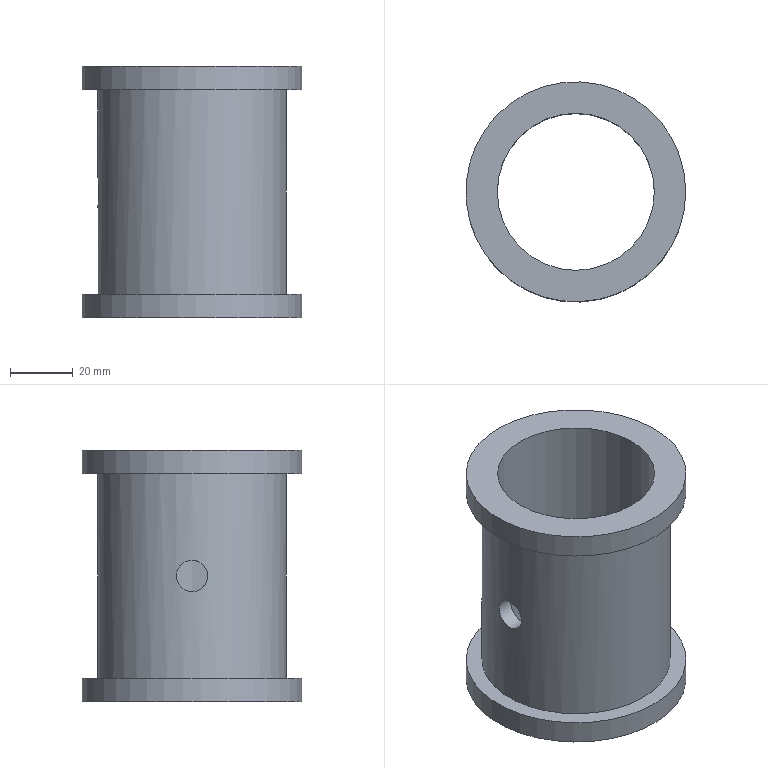Part | NX | features CYLINDER 5, DATUM_CSYS 1 | 1 solid | 9 faces | box 70 x 70 x 80 mm | volume 84036 mm3 | cylinder 5 | plane 4 | commonest cylinder face diameters 70 x2 10 x1 50 x1 60 x1
STEP:
#1=CARTESIAN_POINT('',(-30.,0.,45.));
#2=VERTEX_POINT('',#1);
#3=CARTESIAN_POINT('',(-29.791,-3.922,43.915));
#4=CARTESIAN_POINT('',(-30.104,0.0009284,45.542));
#5=CARTESIAN_POINT('',(-29.792,3.919,43.916));
#6=CARTESIAN_POINT('',(-29.475,5.54,40.005));
#7=CARTESIAN_POINT('',(-29.791,3.919,36.082));
#8=CARTESIAN_POINT('',(-30.104,0.001467,34.46));
#9=CARTESIAN_POINT('',(-29.792,-3.914,36.078));
#10=CARTESIAN_POINT('',(-29.475,-5.541,39.996));
#11=CARTESIAN_POINT('',(-29.791,-3.922,43.915));
#12=CARTESIAN_POINT('',(-30.104,0.0009284,45.542));
#13=CARTESIAN_POINT('',(-29.792,3.919,43.916));
#14=B_SPLINE_CURVE_WITH_KNOTS('',3,(#3,#4,#5,#6,#7,#8,#9,#10,#11,#12,#13),.UNSPECIFIED.,.T.,.F.,(1,1,1,1,1,1,1,1,1,1,1,1,1,1,1),(-0.01174,-0.007829,-0.003914,0.,0.003914,0.007829,0.01174,0.01566,0.01957,0.02349,0.0274,0.03132,0.03523,0.03914,0.04306),.UNSPECIFIED.);
#15=EDGE_CURVE('',#2,#2,#14,.T.);
#16=ORIENTED_EDGE('',*,*,#15,.F.);
#17=EDGE_LOOP('',(#16));
#18=FACE_BOUND('',#17,.T.);
#19=CARTESIAN_POINT('',(-30.,0.,72.5));
#20=VERTEX_POINT('',#19);
#21=CARTESIAN_POINT('',(0.,0.,72.5));
#22=DIRECTION('',(0.,0.,-1.));
#23=DIRECTION('',(-1.,0.,0.));
#24=AXIS2_PLACEMENT_3D('',#21,#22,#23);
#25=CIRCLE('',#24,30.);
#26=EDGE_CURVE('',#20,#20,#25,.F.);
#27=ORIENTED_EDGE('',*,*,#26,.F.);
#28=EDGE_LOOP('',(#27));
#29=FACE_BOUND('',#28,.T.);
#30=CARTESIAN_POINT('',(30.,0.,7.5));
#31=VERTEX_POINT('',#30);
#32=CARTESIAN_POINT('',(0.,0.,7.5));
#33=DIRECTION('',(0.,0.,1.));
#34=DIRECTION('',(1.,0.,0.));
#35=AXIS2_PLACEMENT_3D('',#32,#33,#34);
#36=CIRCLE('',#35,30.);
#37=EDGE_CURVE('',#31,#31,#36,.F.);
#38=ORIENTED_EDGE('',*,*,#37,.F.);
#39=EDGE_LOOP('',(#38));
#40=FACE_BOUND('',#39,.T.);
#41=CARTESIAN_POINT('',(0.,0.,0.));
#42=DIRECTION('',(0.,0.,1.));
#43=DIRECTION('',(1.,0.,0.));
#44=AXIS2_PLACEMENT_3D('',#41,#42,#43);
#45=CYLINDRICAL_SURFACE('',#44,30.);
#46=ADVANCED_FACE('',(#18,#29,#40),#45,.T.);
#47=ORIENTED_EDGE('',*,*,#37,.T.);
#48=EDGE_LOOP('',(#47));
#49=FACE_BOUND('',#48,.T.);
#50=CARTESIAN_POINT('',(35.,0.,7.5));
#51=VERTEX_POINT('',#50);
#52=CARTESIAN_POINT('',(0.,0.,7.5));
#53=DIRECTION('',(0.,0.,-1.));
#54=DIRECTION('',(1.,0.,0.));
#55=AXIS2_PLACEMENT_3D('',#52,#53,#54);
#56=CIRCLE('',#55,35.);
#57=EDGE_CURVE('',#51,#51,#56,.T.);
#58=ORIENTED_EDGE('',*,*,#57,.F.);
#59=EDGE_LOOP('',(#58));
#60=FACE_BOUND('',#59,.T.);
#61=CARTESIAN_POINT('',(0.,0.,7.5));
#62=DIRECTION('',(0.,0.,1.));
#63=DIRECTION('',(1.,0.,0.));
#64=AXIS2_PLACEMENT_3D('',#61,#62,#63);
#65=PLANE('',#64);
#66=ADVANCED_FACE('',(#49,#60),#65,.T.);
#67=ORIENTED_EDGE('',*,*,#57,.T.);
#68=EDGE_LOOP('',(#67));
#69=FACE_BOUND('',#68,.T.);
#70=CARTESIAN_POINT('',(35.,0.,0.));
#71=VERTEX_POINT('',#70);
#72=CARTESIAN_POINT('',(0.,0.,0.));
#73=DIRECTION('',(0.,0.,1.));
#74=DIRECTION('',(1.,0.,0.));
#75=AXIS2_PLACEMENT_3D('',#72,#73,#74);
#76=CIRCLE('',#75,35.);
#77=EDGE_CURVE('',#71,#71,#76,.T.);
#78=ORIENTED_EDGE('',*,*,#77,.T.);
#79=EDGE_LOOP('',(#78));
#80=FACE_BOUND('',#79,.T.);
#81=CARTESIAN_POINT('',(0.,0.,0.));
#82=DIRECTION('',(0.,0.,1.));
#83=DIRECTION('',(1.,0.,0.));
#84=AXIS2_PLACEMENT_3D('',#81,#82,#83);
#85=CYLINDRICAL_SURFACE('',#84,35.);
#86=ADVANCED_FACE('',(#69,#80),#85,.T.);
#87=CARTESIAN_POINT('',(25.,0.,0.));
#88=VERTEX_POINT('',#87);
#89=CARTESIAN_POINT('',(0.,0.,0.));
#90=DIRECTION('',(0.,0.,1.));
#91=DIRECTION('',(1.,0.,0.));
#92=AXIS2_PLACEMENT_3D('',#89,#90,#91);
#93=CIRCLE('',#92,25.);
#94=EDGE_CURVE('',#88,#88,#93,.T.);
#95=ORIENTED_EDGE('',*,*,#94,.T.);
#96=EDGE_LOOP('',(#95));
#97=FACE_BOUND('',#96,.T.);
#98=ORIENTED_EDGE('',*,*,#77,.F.);
#99=EDGE_LOOP('',(#98));
#100=FACE_BOUND('',#99,.T.);
#101=CARTESIAN_POINT('',(0.,0.,0.));
#102=DIRECTION('',(0.,0.,-1.));
#103=DIRECTION('',(-1.,0.,0.));
#104=AXIS2_PLACEMENT_3D('',#101,#102,#103);
#105=PLANE('',#104);
#106=ADVANCED_FACE('',(#97,#100),#105,.T.);
#107=ORIENTED_EDGE('',*,*,#26,.T.);
#108=EDGE_LOOP('',(#107));
#109=FACE_BOUND('',#108,.T.);
#110=CARTESIAN_POINT('',(35.,0.,72.5));
#111=VERTEX_POINT('',#110);
#112=CARTESIAN_POINT('',(0.,0.,72.5));
#113=DIRECTION('',(0.,0.,1.));
#114=DIRECTION('',(1.,0.,0.));
#115=AXIS2_PLACEMENT_3D('',#112,#113,#114);
#116=CIRCLE('',#115,35.);
#117=EDGE_CURVE('',#111,#111,#116,.T.);
#118=ORIENTED_EDGE('',*,*,#117,.F.);
#119=EDGE_LOOP('',(#118));
#120=FACE_BOUND('',#119,.T.);
#121=CARTESIAN_POINT('',(0.,0.,72.5));
#122=DIRECTION('',(0.,0.,-1.));
#123=DIRECTION('',(-1.,0.,0.));
#124=AXIS2_PLACEMENT_3D('',#121,#122,#123);
#125=PLANE('',#124);
#126=ADVANCED_FACE('',(#109,#120),#125,.T.);
#127=ORIENTED_EDGE('',*,*,#117,.T.);
#128=EDGE_LOOP('',(#127));
#129=FACE_BOUND('',#128,.T.);
#130=CARTESIAN_POINT('',(35.,0.,80.));
#131=VERTEX_POINT('',#130);
#132=CARTESIAN_POINT('',(0.,0.,80.));
#133=DIRECTION('',(0.,0.,-1.));
#134=DIRECTION('',(1.,0.,0.));
#135=AXIS2_PLACEMENT_3D('',#132,#133,#134);
#136=CIRCLE('',#135,35.);
#137=EDGE_CURVE('',#131,#131,#136,.T.);
#138=ORIENTED_EDGE('',*,*,#137,.T.);
#139=EDGE_LOOP('',(#138));
#140=FACE_BOUND('',#139,.T.);
#141=CARTESIAN_POINT('',(0.,0.,80.));
#142=DIRECTION('',(0.,0.,-1.));
#143=DIRECTION('',(1.,0.,0.));
#144=AXIS2_PLACEMENT_3D('',#141,#142,#143);
#145=CYLINDRICAL_SURFACE('',#144,35.);
#146=ADVANCED_FACE('',(#129,#140),#145,.T.);
#147=CARTESIAN_POINT('',(25.,0.,80.));
#148=VERTEX_POINT('',#147);
#149=CARTESIAN_POINT('',(0.,0.,80.));
#150=DIRECTION('',(0.,0.,-1.));
#151=DIRECTION('',(1.,0.,0.));
#152=AXIS2_PLACEMENT_3D('',#149,#150,#151);
#153=CIRCLE('',#152,25.);
#154=EDGE_CURVE('',#148,#148,#153,.T.);
#155=ORIENTED_EDGE('',*,*,#154,.T.);
#156=EDGE_LOOP('',(#155));
#157=FACE_BOUND('',#156,.T.);
#158=ORIENTED_EDGE('',*,*,#137,.F.);
#159=EDGE_LOOP('',(#158));
#160=FACE_BOUND('',#159,.T.);
#161=CARTESIAN_POINT('',(0.,0.,80.));
#162=DIRECTION('',(0.,0.,1.));
#163=DIRECTION('',(1.,0.,0.));
#164=AXIS2_PLACEMENT_3D('',#161,#162,#163);
#165=PLANE('',#164);
#166=ADVANCED_FACE('',(#157,#160),#165,.T.);
#167=CARTESIAN_POINT('',(-25.,0.,45.));
#168=VERTEX_POINT('',#167);
#169=CARTESIAN_POINT('',(-24.749,-3.922,43.915));
#170=CARTESIAN_POINT('',(-25.125,0.0008753,45.542));
#171=CARTESIAN_POINT('',(-24.75,3.919,43.916));
#172=CARTESIAN_POINT('',(-24.367,5.541,40.005));
#173=CARTESIAN_POINT('',(-24.75,3.919,36.082));
#174=CARTESIAN_POINT('',(-25.125,0.001797,34.46));
#175=CARTESIAN_POINT('',(-24.751,-3.914,36.078));
#176=CARTESIAN_POINT('',(-24.367,-5.541,39.997));
#177=CARTESIAN_POINT('',(-24.749,-3.922,43.915));
#178=CARTESIAN_POINT('',(-25.125,0.0008753,45.542));
#179=CARTESIAN_POINT('',(-24.75,3.919,43.916));
#180=B_SPLINE_CURVE_WITH_KNOTS('',3,(#169,#170,#171,#172,#173,#174,#175,#176,#177,#178,#179),.UNSPECIFIED.,.T.,.F.,(1,1,1,1,1,1,1,1,1,1,1,1,1,1,1),(-0.01175,-0.007835,-0.003917,0.,0.003917,0.007835,0.01175,0.01567,0.01959,0.0235,0.02742,0.03134,0.03526,0.03917,0.04309),.UNSPECIFIED.);
#181=EDGE_CURVE('',#168,#168,#180,.T.);
#182=ORIENTED_EDGE('',*,*,#181,.T.);
#183=EDGE_LOOP('',(#182));
#184=FACE_BOUND('',#183,.T.);
#185=ORIENTED_EDGE('',*,*,#154,.F.);
#186=EDGE_LOOP('',(#185));
#187=FACE_BOUND('',#186,.T.);
#188=ORIENTED_EDGE('',*,*,#94,.F.);
#189=EDGE_LOOP('',(#188));
#190=FACE_BOUND('',#189,.T.);
#191=CARTESIAN_POINT('',(0.,0.,0.));
#192=DIRECTION('',(0.,0.,1.));
#193=DIRECTION('',(1.,0.,0.));
#194=AXIS2_PLACEMENT_3D('',#191,#192,#193);
#195=CYLINDRICAL_SURFACE('',#194,25.);
#196=ADVANCED_FACE('',(#184,#187,#190),#195,.F.);
#197=ORIENTED_EDGE('',*,*,#15,.T.);
#198=EDGE_LOOP('',(#197));
#199=FACE_BOUND('',#198,.T.);
#200=ORIENTED_EDGE('',*,*,#181,.F.);
#201=EDGE_LOOP('',(#200));
#202=FACE_BOUND('',#201,.T.);
#203=CARTESIAN_POINT('',(0.,0.,40.));
#204=DIRECTION('',(-1.,0.,0.));
#205=DIRECTION('',(0.,0.,1.));
#206=AXIS2_PLACEMENT_3D('',#203,#204,#205);
#207=CYLINDRICAL_SURFACE('',#206,5.);
#208=ADVANCED_FACE('',(#199,#202),#207,.F.);
#209=CLOSED_SHELL('',(#46,#66,#86,#106,#126,#146,#166,#196,#208));
#210=MANIFOLD_SOLID_BREP('',#209);
#211=(LENGTH_UNIT()NAMED_UNIT(*)SI_UNIT(.MILLI.,.METRE.));
#212=UNCERTAINTY_MEASURE_WITH_UNIT(LENGTH_MEASURE(0.0508),#211,'','');
#213=(NAMED_UNIT(*)PLANE_ANGLE_UNIT()SI_UNIT($,.RADIAN.));
#214=(NAMED_UNIT(*)SI_UNIT($,.STERADIAN.)SOLID_ANGLE_UNIT());
#215=(GEOMETRIC_REPRESENTATION_CONTEXT(3)GLOBAL_UNCERTAINTY_ASSIGNED_CONTEXT((#212))GLOBAL_UNIT_ASSIGNED_CONTEXT((#211,#213,#214))REPRESENTATION_CONTEXT('',''));
#216=ADVANCED_BREP_SHAPE_REPRESENTATION('',(#210),#215);